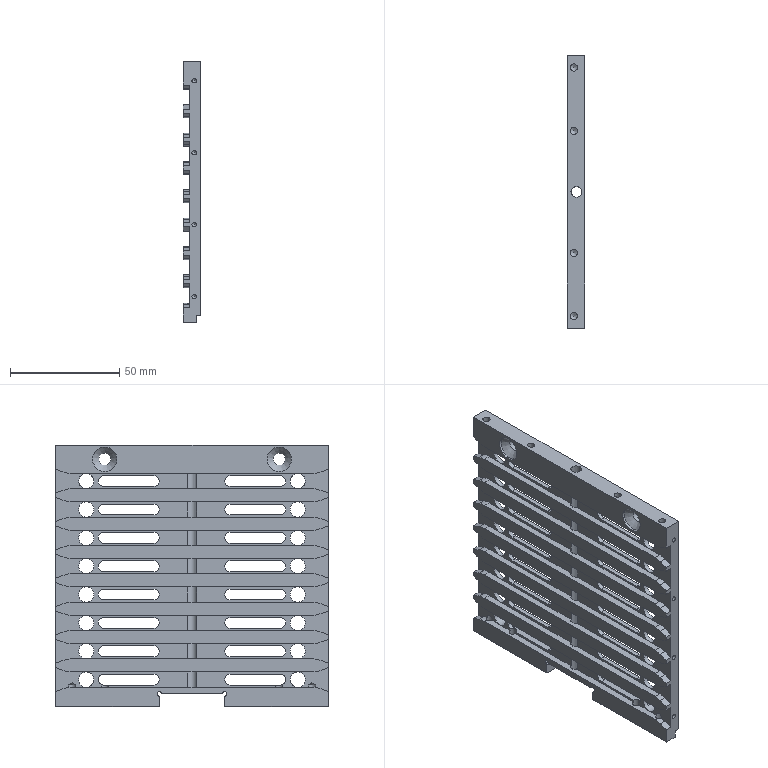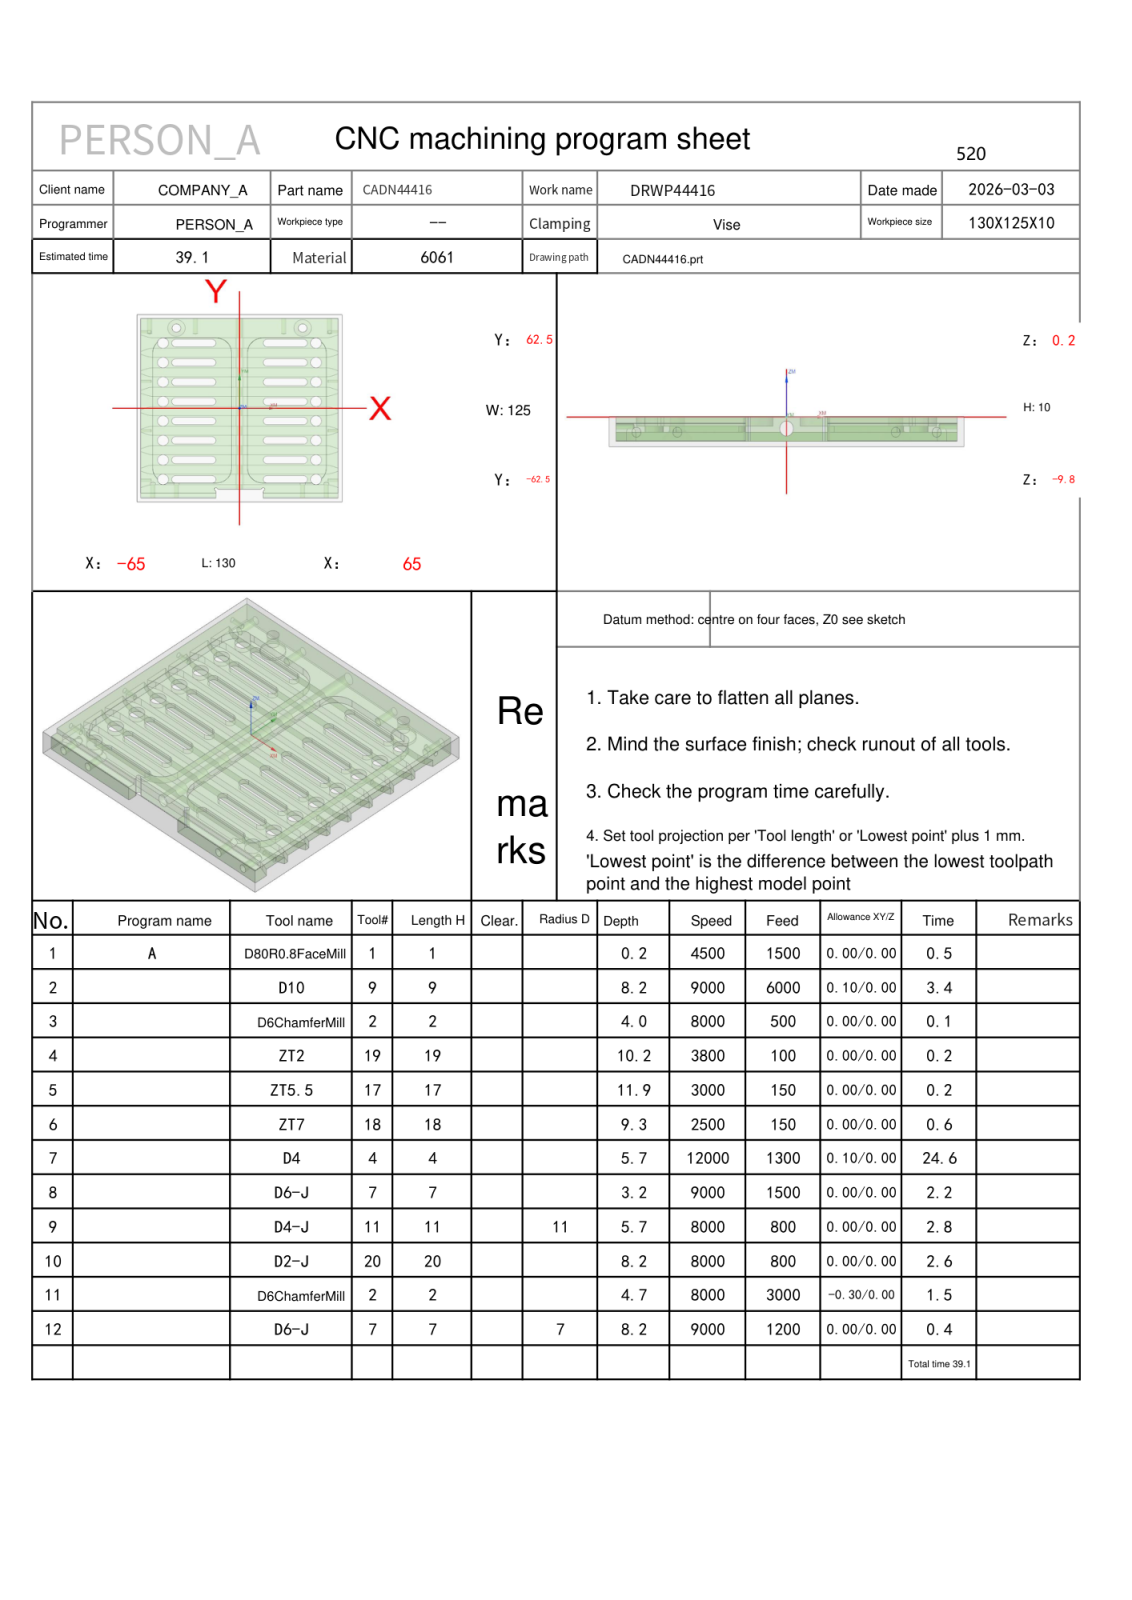NC program | NX | posted by the shop | part box 8 x 125 x 120 mm
Lines 826 to 1740 of 11100:
N7 T04 M06
(D4  D=4. R=0. H=04 ce=0.10 di=0.00)
G00 G90 G54 X29. Y-34.1 M03 S12000
G43 H04 Z30.
M08
Z-2.5
G01 X17.5 Z-2.536 F800.
G03 X17.1 Y-34.5 Z-2.538 I0.0 J-.4
X17.5 Y-34.9 Z-2.539 I.4 J0.0
G01 X40.5 Z-2.611
G03 X40.9 Y-34.5 Z-2.613 I0.0 J.4
X40.5 Y-34.1 Z-2.614 I-.4 J0.0
G01 X17.5 Z-2.686
G03 X17.1 Y-34.5 Z-2.688 I0.0 J-.4
X17.5 Y-34.9 Z-2.689 I.4 J0.0
G01 X40.5 Z-2.761
G03 X40.9 Y-34.5 Z-2.763 I0.0 J.4
X40.5 Y-34.1 Z-2.764 I-.4 J0.0
G01 X17.5 Z-2.836
G03 X17.1 Y-34.5 Z-2.838 I0.0 J-.4
X17.5 Y-34.9 Z-2.839 I.4 J0.0
G01 X40.5 Z-2.911
G03 X40.9 Y-34.5 Z-2.913 I0.0 J.4
X40.5 Y-34.1 Z-2.914 I-.4 J0.0
G01 X17.5 Z-2.986
G03 X17.1 Y-34.5 Z-2.988 I0.0 J-.4
X17.5 Y-34.9 Z-2.989 I.4 J0.0
G01 X40.5 Z-3.061
G03 X40.9 Y-34.5 Z-3.063 I0.0 J.4
X40.5 Y-34.1 Z-3.064 I-.4 J0.0
G01 X17.5 Z-3.136
G03 X17.1 Y-34.5 Z-3.138 I0.0 J-.4
X17.5 Y-34.9 Z-3.139 I.4 J0.0
G01 X40.5 Z-3.211
G03 X40.9 Y-34.5 Z-3.213 I0.0 J.4
X40.5 Y-34.1 Z-3.214 I-.4 J0.0
G01 X17.5 Z-3.286
G03 X17.1 Y-34.5 Z-3.288 I0.0 J-.4
X17.5 Y-34.9 Z-3.289 I.4 J0.0
G01 X40.5 Z-3.361
G03 X40.9 Y-34.5 Z-3.363 I0.0 J.4
X40.5 Y-34.1 Z-3.364 I-.4 J0.0
G01 X17.5 Z-3.436
G03 X17.1 Y-34.5 Z-3.438 I0.0 J-.4
X17.5 Y-34.9 Z-3.439 I.4 J0.0
G01 X40.5 Z-3.511
G03 X40.9 Y-34.5 Z-3.513 I0.0 J.4
X40.5 Y-34.1 Z-3.514 I-.4 J0.0
G01 X17.5 Z-3.586
G03 X17.1 Y-34.5 Z-3.588 I0.0 J-.4
X17.5 Y-34.9 Z-3.589 I.4 J0.0
G01 X40.5 Z-3.661
G03 X40.9 Y-34.5 Z-3.663 I0.0 J.4
X40.5 Y-34.1 Z-3.664 I-.4 J0.0
G01 X17.5 Z-3.736
G03 X17.1 Y-34.5 Z-3.738 I0.0 J-.4
X17.5 Y-34.9 Z-3.739 I.4 J0.0
G01 X40.5 Z-3.811
G03 X40.9 Y-34.5 Z-3.813 I0.0 J.4
X40.5 Y-34.1 Z-3.814 I-.4 J0.0
G01 X17.5 Z-3.886
G03 X17.1 Y-34.5 Z-3.888 I0.0 J-.4
X17.5 Y-34.9 Z-3.889 I.4 J0.0
G01 X40.5 Z-3.961
G03 X40.9 Y-34.5 Z-3.963 I0.0 J.4
X40.5 Y-34.1 Z-3.964 I-.4 J0.0
G01 X17.5 Z-4.036
G03 X17.1 Y-34.5 Z-4.038 I0.0 J-.4
X17.5 Y-34.9 Z-4.039 I.4 J0.0
G01 X40.5 Z-4.111
G03 X40.9 Y-34.5 Z-4.113 I0.0 J.4
X40.5 Y-34.1 Z-4.114 I-.4 J0.0
G01 X17.5 Z-4.186
G03 X17.1 Y-34.5 Z-4.188 I0.0 J-.4
X17.5 Y-34.9 Z-4.189 I.4 J0.0
G01 X40.5 Z-4.261
G03 X40.9 Y-34.5 Z-4.263 I0.0 J.4
X40.5 Y-34.1 Z-4.264 I-.4 J0.0
G01 X17.5 Z-4.336
G03 X17.1 Y-34.5 Z-4.338 I0.0 J-.4
X17.5 Y-34.9 Z-4.339 I.4 J0.0
G01 X40.5 Z-4.411
G03 X40.9 Y-34.5 Z-4.413 I0.0 J.4
X40.5 Y-34.1 Z-4.414 I-.4 J0.0
G01 X17.5 Z-4.486
G03 X17.1 Y-34.5 Z-4.488 I0.0 J-.4
X17.5 Y-34.9 Z-4.489 I.4 J0.0
G01 X40.5 Z-4.561
G03 X40.9 Y-34.5 Z-4.563 I0.0 J.4
X40.5 Y-34.1 Z-4.564 I-.4 J0.0
G01 X17.5 Z-4.636
G03 X17.1 Y-34.5 Z-4.638 I0.0 J-.4
X17.5 Y-34.9 Z-4.639 I.4 J0.0
G01 X40.5 Z-4.711
G03 X40.9 Y-34.5 Z-4.713 I0.0 J.4
X40.5 Y-34.1 Z-4.714 I-.4 J0.0
G01 X17.5 Z-4.786
G03 X17.1 Y-34.5 Z-4.788 I0.0 J-.4
X17.5 Y-34.9 Z-4.789 I.4 J0.0
G01 X40.5 Z-4.861
G03 X40.9 Y-34.5 Z-4.863 I0.0 J.4
X40.5 Y-34.1 Z-4.864 I-.4 J0.0
G01 X17.5 Z-4.936
G03 X17.1 Y-34.5 Z-4.938 I0.0 J-.4
X17.5 Y-34.9 Z-4.939 I.4 J0.0
G01 X40.5 Z-5.011
G03 X40.9 Y-34.5 Z-5.013 I0.0 J.4
X40.5 Y-34.1 Z-5.014 I-.4 J0.0
G01 X17.5 Z-5.086
G03 X17.1 Y-34.5 Z-5.088 I0.0 J-.4
X17.5 Y-34.9 Z-5.089 I.4 J0.0
G01 X40.5 Z-5.161
G03 X40.9 Y-34.5 Z-5.163 I0.0 J.4
X40.5 Y-34.1 Z-5.164 I-.4 J0.0
G01 X17.5 Z-5.236
G03 X17.1 Y-34.5 Z-5.238 I0.0 J-.4
X17.5 Y-34.9 Z-5.239 I.4 J0.0
G01 X40.5 Z-5.311
G03 X40.9 Y-34.5 Z-5.313 I0.0 J.4
X40.5 Y-34.1 Z-5.314 I-.4 J0.0
G01 X17.5 Z-5.386
G03 X17.1 Y-34.5 Z-5.388 I0.0 J-.4
X17.5 Y-34.9 Z-5.389 I.4 J0.0
G01 X40.5 Z-5.461
G03 X40.9 Y-34.5 Z-5.463 I0.0 J.4
X40.5 Y-34.1 Z-5.464 I-.4 J0.0
G01 X29. Z-5.5
X17.5
G03 X17.1 Y-34.5 I0.0 J-.4
X17.5 Y-34.9 I.4 J0.0
G01 X40.5
G03 X40.9 Y-34.5 I0.0 J.4
X40.5 Y-34.1 I-.4 J0.0
G01 X29.
X28.5
Z-4.5
G00 Z30.
X29. Y-21.9
Z-2.5
G01 X40.5 Z-2.536
G03 X40.9 Y-21.5 Z-2.538 I0.0 J.4
X40.5 Y-21.1 Z-2.539 I-.4 J0.0
G01 X17.5 Z-2.611
G03 X17.1 Y-21.5 Z-2.613 I0.0 J-.4
X17.5 Y-21.9 Z-2.614 I.4 J0.0
G01 X40.5 Z-2.686
G03 X40.9 Y-21.5 Z-2.688 I0.0 J.4
X40.5 Y-21.1 Z-2.689 I-.4 J0.0
G01 X17.5 Z-2.761
G03 X17.1 Y-21.5 Z-2.763 I0.0 J-.4
X17.5 Y-21.9 Z-2.764 I.4 J0.0
G01 X40.5 Z-2.836
G03 X40.9 Y-21.5 Z-2.838 I0.0 J.4
X40.5 Y-21.1 Z-2.839 I-.4 J0.0
G01 X17.5 Z-2.911
G03 X17.1 Y-21.5 Z-2.913 I0.0 J-.4
X17.5 Y-21.9 Z-2.914 I.4 J0.0
G01 X40.5 Z-2.986
G03 X40.9 Y-21.5 Z-2.988 I0.0 J.4
X40.5 Y-21.1 Z-2.989 I-.4 J0.0
G01 X17.5 Z-3.061
G03 X17.1 Y-21.5 Z-3.063 I0.0 J-.4
X17.5 Y-21.9 Z-3.064 I.4 J0.0
G01 X40.5 Z-3.136
G03 X40.9 Y-21.5 Z-3.138 I0.0 J.4
X40.5 Y-21.1 Z-3.139 I-.4 J0.0
G01 X17.5 Z-3.211
G03 X17.1 Y-21.5 Z-3.213 I0.0 J-.4
X17.5 Y-21.9 Z-3.214 I.4 J0.0
G01 X40.5 Z-3.286
G03 X40.9 Y-21.5 Z-3.288 I0.0 J.4
X40.5 Y-21.1 Z-3.289 I-.4 J0.0
G01 X17.5 Z-3.361
G03 X17.1 Y-21.5 Z-3.363 I0.0 J-.4
X17.5 Y-21.9 Z-3.364 I.4 J0.0
G01 X40.5 Z-3.436
G03 X40.9 Y-21.5 Z-3.438 I0.0 J.4
X40.5 Y-21.1 Z-3.439 I-.4 J0.0
G01 X17.5 Z-3.511
G03 X17.1 Y-21.5 Z-3.513 I0.0 J-.4
X17.5 Y-21.9 Z-3.514 I.4 J0.0
G01 X40.5 Z-3.586
G03 X40.9 Y-21.5 Z-3.588 I0.0 J.4
X40.5 Y-21.1 Z-3.589 I-.4 J0.0
G01 X17.5 Z-3.661
G03 X17.1 Y-21.5 Z-3.663 I0.0 J-.4
X17.5 Y-21.9 Z-3.664 I.4 J0.0
G01 X40.5 Z-3.736
G03 X40.9 Y-21.5 Z-3.738 I0.0 J.4
X40.5 Y-21.1 Z-3.739 I-.4 J0.0
G01 X17.5 Z-3.811
G03 X17.1 Y-21.5 Z-3.813 I0.0 J-.4
X17.5 Y-21.9 Z-3.814 I.4 J0.0
G01 X40.5 Z-3.886
G03 X40.9 Y-21.5 Z-3.888 I0.0 J.4
X40.5 Y-21.1 Z-3.889 I-.4 J0.0
G01 X17.5 Z-3.961
G03 X17.1 Y-21.5 Z-3.963 I0.0 J-.4
X17.5 Y-21.9 Z-3.964 I.4 J0.0
G01 X40.5 Z-4.036
G03 X40.9 Y-21.5 Z-4.038 I0.0 J.4
X40.5 Y-21.1 Z-4.039 I-.4 J0.0
G01 X17.5 Z-4.111
G03 X17.1 Y-21.5 Z-4.113 I0.0 J-.4
X17.5 Y-21.9 Z-4.114 I.4 J0.0
G01 X40.5 Z-4.186
G03 X40.9 Y-21.5 Z-4.188 I0.0 J.4
X40.5 Y-21.1 Z-4.189 I-.4 J0.0
G01 X17.5 Z-4.261
G03 X17.1 Y-21.5 Z-4.263 I0.0 J-.4
X17.5 Y-21.9 Z-4.264 I.4 J0.0
G01 X40.5 Z-4.336
G03 X40.9 Y-21.5 Z-4.338 I0.0 J.4
X40.5 Y-21.1 Z-4.339 I-.4 J0.0
G01 X17.5 Z-4.411
G03 X17.1 Y-21.5 Z-4.413 I0.0 J-.4
X17.5 Y-21.9 Z-4.414 I.4 J0.0
G01 X40.5 Z-4.486
G03 X40.9 Y-21.5 Z-4.488 I0.0 J.4
X40.5 Y-21.1 Z-4.489 I-.4 J0.0
G01 X17.5 Z-4.561
G03 X17.1 Y-21.5 Z-4.563 I0.0 J-.4
X17.5 Y-21.9 Z-4.564 I.4 J0.0
G01 X40.5 Z-4.636
G03 X40.9 Y-21.5 Z-4.638 I0.0 J.4
X40.5 Y-21.1 Z-4.639 I-.4 J0.0
G01 X17.5 Z-4.711
G03 X17.1 Y-21.5 Z-4.713 I0.0 J-.4
X17.5 Y-21.9 Z-4.714 I.4 J0.0
G01 X40.5 Z-4.786
G03 X40.9 Y-21.5 Z-4.788 I0.0 J.4
X40.5 Y-21.1 Z-4.789 I-.4 J0.0
G01 X17.5 Z-4.861
G03 X17.1 Y-21.5 Z-4.863 I0.0 J-.4
X17.5 Y-21.9 Z-4.864 I.4 J0.0
G01 X40.5 Z-4.936
G03 X40.9 Y-21.5 Z-4.938 I0.0 J.4
X40.5 Y-21.1 Z-4.939 I-.4 J0.0
G01 X17.5 Z-5.011
G03 X17.1 Y-21.5 Z-5.013 I0.0 J-.4
X17.5 Y-21.9 Z-5.014 I.4 J0.0
G01 X40.5 Z-5.086
G03 X40.9 Y-21.5 Z-5.088 I0.0 J.4
X40.5 Y-21.1 Z-5.089 I-.4 J0.0
G01 X17.5 Z-5.161
G03 X17.1 Y-21.5 Z-5.163 I0.0 J-.4
X17.5 Y-21.9 Z-5.164 I.4 J0.0
G01 X40.5 Z-5.236
G03 X40.9 Y-21.5 Z-5.238 I0.0 J.4
X40.5 Y-21.1 Z-5.239 I-.4 J0.0
G01 X17.5 Z-5.311
G03 X17.1 Y-21.5 Z-5.313 I0.0 J-.4
X17.5 Y-21.9 Z-5.314 I.4 J0.0
G01 X40.5 Z-5.386
G03 X40.9 Y-21.5 Z-5.388 I0.0 J.4
X40.5 Y-21.1 Z-5.389 I-.4 J0.0
G01 X17.5 Z-5.461
G03 X17.1 Y-21.5 Z-5.463 I0.0 J-.4
X17.5 Y-21.9 Z-5.464 I.4 J0.0
G01 X29. Z-5.5
X40.5
G03 X40.9 Y-21.5 I0.0 J.4
X40.5 Y-21.1 I-.4 J0.0
G01 X17.5
G03 X17.1 Y-21.5 I0.0 J-.4
X17.5 Y-21.9 I.4 J0.0
G01 X29.
X29.5
Z-4.5
G00 Z30.
X29. Y-8.9
Z-2.5
G01 X40.5 Z-2.536
G03 X40.9 Y-8.5 Z-2.538 I0.0 J.4
X40.5 Y-8.1 Z-2.539 I-.4 J0.0
G01 X17.5 Z-2.611
G03 X17.1 Y-8.5 Z-2.613 I0.0 J-.4
X17.5 Y-8.9 Z-2.614 I.4 J0.0
G01 X40.5 Z-2.686
G03 X40.9 Y-8.5 Z-2.688 I0.0 J.4
X40.5 Y-8.1 Z-2.689 I-.4 J0.0
G01 X17.5 Z-2.761
G03 X17.1 Y-8.5 Z-2.763 I0.0 J-.4
X17.5 Y-8.9 Z-2.764 I.4 J0.0
G01 X40.5 Z-2.836
G03 X40.9 Y-8.5 Z-2.838 I0.0 J.4
X40.5 Y-8.1 Z-2.839 I-.4 J0.0
G01 X17.5 Z-2.911
G03 X17.1 Y-8.5 Z-2.913 I0.0 J-.4
X17.5 Y-8.9 Z-2.914 I.4 J0.0
G01 X40.5 Z-2.986
G03 X40.9 Y-8.5 Z-2.988 I0.0 J.4
X40.5 Y-8.1 Z-2.989 I-.4 J0.0
G01 X17.5 Z-3.061
G03 X17.1 Y-8.5 Z-3.063 I0.0 J-.4
X17.5 Y-8.9 Z-3.064 I.4 J0.0
G01 X40.5 Z-3.136
G03 X40.9 Y-8.5 Z-3.138 I0.0 J.4
X40.5 Y-8.1 Z-3.139 I-.4 J0.0
G01 X17.5 Z-3.211
G03 X17.1 Y-8.5 Z-3.213 I0.0 J-.4
X17.5 Y-8.9 Z-3.214 I.4 J0.0
G01 X40.5 Z-3.286
G03 X40.9 Y-8.5 Z-3.288 I0.0 J.4
X40.5 Y-8.1 Z-3.289 I-.4 J0.0
G01 X17.5 Z-3.361
G03 X17.1 Y-8.5 Z-3.363 I0.0 J-.4
X17.5 Y-8.9 Z-3.364 I.4 J0.0
G01 X40.5 Z-3.436
G03 X40.9 Y-8.5 Z-3.438 I0.0 J.4
X40.5 Y-8.1 Z-3.439 I-.4 J0.0
G01 X17.5 Z-3.511
G03 X17.1 Y-8.5 Z-3.513 I0.0 J-.4
X17.5 Y-8.9 Z-3.514 I.4 J0.0
G01 X40.5 Z-3.586
G03 X40.9 Y-8.5 Z-3.588 I0.0 J.4
X40.5 Y-8.1 Z-3.589 I-.4 J0.0
G01 X17.5 Z-3.661
G03 X17.1 Y-8.5 Z-3.663 I0.0 J-.4
X17.5 Y-8.9 Z-3.664 I.4 J0.0
G01 X40.5 Z-3.736
G03 X40.9 Y-8.5 Z-3.738 I0.0 J.4
X40.5 Y-8.1 Z-3.739 I-.4 J0.0
G01 X17.5 Z-3.811
G03 X17.1 Y-8.5 Z-3.813 I0.0 J-.4
X17.5 Y-8.9 Z-3.814 I.4 J0.0
G01 X40.5 Z-3.886
G03 X40.9 Y-8.5 Z-3.888 I0.0 J.4
X40.5 Y-8.1 Z-3.889 I-.4 J0.0
G01 X17.5 Z-3.961
G03 X17.1 Y-8.5 Z-3.963 I0.0 J-.4
X17.5 Y-8.9 Z-3.964 I.4 J0.0
G01 X40.5 Z-4.036
G03 X40.9 Y-8.5 Z-4.038 I0.0 J.4
X40.5 Y-8.1 Z-4.039 I-.4 J0.0
G01 X17.5 Z-4.111
G03 X17.1 Y-8.5 Z-4.113 I0.0 J-.4
X17.5 Y-8.9 Z-4.114 I.4 J0.0
G01 X40.5 Z-4.186
G03 X40.9 Y-8.5 Z-4.188 I0.0 J.4
X40.5 Y-8.1 Z-4.189 I-.4 J0.0
G01 X17.5 Z-4.261
G03 X17.1 Y-8.5 Z-4.263 I0.0 J-.4
X17.5 Y-8.9 Z-4.264 I.4 J0.0
G01 X40.5 Z-4.336
G03 X40.9 Y-8.5 Z-4.338 I0.0 J.4
X40.5 Y-8.1 Z-4.339 I-.4 J0.0
G01 X17.5 Z-4.411
G03 X17.1 Y-8.5 Z-4.413 I0.0 J-.4
X17.5 Y-8.9 Z-4.414 I.4 J0.0
G01 X40.5 Z-4.486
G03 X40.9 Y-8.5 Z-4.488 I0.0 J.4
X40.5 Y-8.1 Z-4.489 I-.4 J0.0
G01 X17.5 Z-4.561
G03 X17.1 Y-8.5 Z-4.563 I0.0 J-.4
X17.5 Y-8.9 Z-4.564 I.4 J0.0
G01 X40.5 Z-4.636
G03 X40.9 Y-8.5 Z-4.638 I0.0 J.4
X40.5 Y-8.1 Z-4.639 I-.4 J0.0
G01 X17.5 Z-4.711
G03 X17.1 Y-8.5 Z-4.713 I0.0 J-.4
X17.5 Y-8.9 Z-4.714 I.4 J0.0
G01 X40.5 Z-4.786
G03 X40.9 Y-8.5 Z-4.788 I0.0 J.4
X40.5 Y-8.1 Z-4.789 I-.4 J0.0
G01 X17.5 Z-4.861
G03 X17.1 Y-8.5 Z-4.863 I0.0 J-.4
X17.5 Y-8.9 Z-4.864 I.4 J0.0
G01 X40.5 Z-4.936
G03 X40.9 Y-8.5 Z-4.938 I0.0 J.4
X40.5 Y-8.1 Z-4.939 I-.4 J0.0
G01 X17.5 Z-5.011
G03 X17.1 Y-8.5 Z-5.013 I0.0 J-.4
X17.5 Y-8.9 Z-5.014 I.4 J0.0
G01 X40.5 Z-5.086
G03 X40.9 Y-8.5 Z-5.088 I0.0 J.4
X40.5 Y-8.1 Z-5.089 I-.4 J0.0
G01 X17.5 Z-5.161
G03 X17.1 Y-8.5 Z-5.163 I0.0 J-.4
X17.5 Y-8.9 Z-5.164 I.4 J0.0
G01 X40.5 Z-5.236
G03 X40.9 Y-8.5 Z-5.238 I0.0 J.4
X40.5 Y-8.1 Z-5.239 I-.4 J0.0
G01 X17.5 Z-5.311
G03 X17.1 Y-8.5 Z-5.313 I0.0 J-.4
X17.5 Y-8.9 Z-5.314 I.4 J0.0
G01 X40.5 Z-5.386
G03 X40.9 Y-8.5 Z-5.388 I0.0 J.4
X40.5 Y-8.1 Z-5.389 I-.4 J0.0
G01 X17.5 Z-5.461
G03 X17.1 Y-8.5 Z-5.463 I0.0 J-.4
X17.5 Y-8.9 Z-5.464 I.4 J0.0
G01 X29. Z-5.5
X40.5
G03 X40.9 Y-8.5 I0.0 J.4
X40.5 Y-8.1 I-.4 J0.0
G01 X17.5
G03 X17.1 Y-8.5 I0.0 J-.4
X17.5 Y-8.9 I.4 J0.0
G01 X29.
X29.5
Z-4.5
G00 Z30.
X29. Y4.9
Z-2.5
G01 X17.5 Z-2.536
G03 X17.1 Y4.5 Z-2.538 I0.0 J-.4
X17.5 Y4.1 Z-2.539 I.4 J0.0
G01 X40.5 Z-2.611
G03 X40.9 Y4.5 Z-2.613 I0.0 J.4
X40.5 Y4.9 Z-2.614 I-.4 J0.0
G01 X17.5 Z-2.686
G03 X17.1 Y4.5 Z-2.688 I0.0 J-.4
X17.5 Y4.1 Z-2.689 I.4 J0.0
G01 X40.5 Z-2.761
G03 X40.9 Y4.5 Z-2.763 I0.0 J.4
X40.5 Y4.9 Z-2.764 I-.4 J0.0
G01 X17.5 Z-2.836
G03 X17.1 Y4.5 Z-2.838 I0.0 J-.4
X17.5 Y4.1 Z-2.839 I.4 J0.0
G01 X40.5 Z-2.911
G03 X40.9 Y4.5 Z-2.913 I0.0 J.4
X40.5 Y4.9 Z-2.914 I-.4 J0.0
G01 X17.5 Z-2.986
G03 X17.1 Y4.5 Z-2.988 I0.0 J-.4
X17.5 Y4.1 Z-2.989 I.4 J0.0
G01 X40.5 Z-3.061
G03 X40.9 Y4.5 Z-3.063 I0.0 J.4
X40.5 Y4.9 Z-3.064 I-.4 J0.0
G01 X17.5 Z-3.136
G03 X17.1 Y4.5 Z-3.138 I0.0 J-.4
X17.5 Y4.1 Z-3.139 I.4 J0.0
G01 X40.5 Z-3.211
G03 X40.9 Y4.5 Z-3.213 I0.0 J.4
X40.5 Y4.9 Z-3.214 I-.4 J0.0
G01 X17.5 Z-3.286
G03 X17.1 Y4.5 Z-3.288 I0.0 J-.4
X17.5 Y4.1 Z-3.289 I.4 J0.0
G01 X40.5 Z-3.361
G03 X40.9 Y4.5 Z-3.363 I0.0 J.4
X40.5 Y4.9 Z-3.364 I-.4 J0.0
G01 X17.5 Z-3.436
G03 X17.1 Y4.5 Z-3.438 I0.0 J-.4
X17.5 Y4.1 Z-3.439 I.4 J0.0
G01 X40.5 Z-3.511
G03 X40.9 Y4.5 Z-3.513 I0.0 J.4
X40.5 Y4.9 Z-3.514 I-.4 J0.0
G01 X17.5 Z-3.586
G03 X17.1 Y4.5 Z-3.588 I0.0 J-.4
X17.5 Y4.1 Z-3.589 I.4 J0.0
G01 X40.5 Z-3.661
G03 X40.9 Y4.5 Z-3.663 I0.0 J.4
X40.5 Y4.9 Z-3.664 I-.4 J0.0
G01 X17.5 Z-3.736
G03 X17.1 Y4.5 Z-3.738 I0.0 J-.4
X17.5 Y4.1 Z-3.739 I.4 J0.0
G01 X40.5 Z-3.811
G03 X40.9 Y4.5 Z-3.813 I0.0 J.4
X40.5 Y4.9 Z-3.814 I-.4 J0.0
G01 X17.5 Z-3.886
G03 X17.1 Y4.5 Z-3.888 I0.0 J-.4
X17.5 Y4.1 Z-3.889 I.4 J0.0
G01 X40.5 Z-3.961
G03 X40.9 Y4.5 Z-3.963 I0.0 J.4
X40.5 Y4.9 Z-3.964 I-.4 J0.0
G01 X17.5 Z-4.036
G03 X17.1 Y4.5 Z-4.038 I0.0 J-.4
X17.5 Y4.1 Z-4.039 I.4 J0.0
G01 X40.5 Z-4.111
G03 X40.9 Y4.5 Z-4.113 I0.0 J.4
X40.5 Y4.9 Z-4.114 I-.4 J0.0
G01 X17.5 Z-4.186
G03 X17.1 Y4.5 Z-4.188 I0.0 J-.4
X17.5 Y4.1 Z-4.189 I.4 J0.0
G01 X40.5 Z-4.261
G03 X40.9 Y4.5 Z-4.263 I0.0 J.4
X40.5 Y4.9 Z-4.264 I-.4 J0.0
G01 X17.5 Z-4.336
G03 X17.1 Y4.5 Z-4.338 I0.0 J-.4
X17.5 Y4.1 Z-4.339 I.4 J0.0
G01 X40.5 Z-4.411
G03 X40.9 Y4.5 Z-4.413 I0.0 J.4
X40.5 Y4.9 Z-4.414 I-.4 J0.0
G01 X17.5 Z-4.486
G03 X17.1 Y4.5 Z-4.488 I0.0 J-.4
X17.5 Y4.1 Z-4.489 I.4 J0.0
G01 X40.5 Z-4.561
G03 X40.9 Y4.5 Z-4.563 I0.0 J.4
X40.5 Y4.9 Z-4.564 I-.4 J0.0
G01 X17.5 Z-4.636
G03 X17.1 Y4.5 Z-4.638 I0.0 J-.4
X17.5 Y4.1 Z-4.639 I.4 J0.0
G01 X40.5 Z-4.711
G03 X40.9 Y4.5 Z-4.713 I0.0 J.4
X40.5 Y4.9 Z-4.714 I-.4 J0.0
G01 X17.5 Z-4.786
G03 X17.1 Y4.5 Z-4.788 I0.0 J-.4
X17.5 Y4.1 Z-4.789 I.4 J0.0
G01 X40.5 Z-4.861
G03 X40.9 Y4.5 Z-4.863 I0.0 J.4
X40.5 Y4.9 Z-4.864 I-.4 J0.0
G01 X17.5 Z-4.936
G03 X17.1 Y4.5 Z-4.938 I0.0 J-.4
X17.5 Y4.1 Z-4.939 I.4 J0.0
G01 X40.5 Z-5.011
G03 X40.9 Y4.5 Z-5.013 I0.0 J.4
X40.5 Y4.9 Z-5.014 I-.4 J0.0
G01 X17.5 Z-5.086
G03 X17.1 Y4.5 Z-5.088 I0.0 J-.4
X17.5 Y4.1 Z-5.089 I.4 J0.0
G01 X40.5 Z-5.161
G03 X40.9 Y4.5 Z-5.163 I0.0 J.4
X40.5 Y4.9 Z-5.164 I-.4 J0.0
G01 X17.5 Z-5.236
G03 X17.1 Y4.5 Z-5.238 I0.0 J-.4
X17.5 Y4.1 Z-5.239 I.4 J0.0
G01 X40.5 Z-5.311
G03 X40.9 Y4.5 Z-5.313 I0.0 J.4
X40.5 Y4.9 Z-5.314 I-.4 J0.0
G01 X17.5 Z-5.386
G03 X17.1 Y4.5 Z-5.388 I0.0 J-.4
X17.5 Y4.1 Z-5.389 I.4 J0.0
G01 X40.5 Z-5.461
G03 X40.9 Y4.5 Z-5.463 I0.0 J.4
X40.5 Y4.9 Z-5.464 I-.4 J0.0
G01 X29. Z-5.5
X17.5
G03 X17.1 Y4.5 I0.0 J-.4
X17.5 Y4.1 I.4 J0.0
G01 X40.5
G03 X40.9 Y4.5 I0.0 J.4
X40.5 Y4.9 I-.4 J0.0
G01 X29.
X28.5
Z-4.5
G00 Z30.
X29. Y17.1
Z-2.5
G01 X40.5 Z-2.536
G03 X40.9 Y17.5 Z-2.538 I0.0 J.4
X40.5 Y17.9 Z-2.539 I-.4 J0.0
G01 X17.5 Z-2.611
G03 X17.1 Y17.5 Z-2.613 I0.0 J-.4
X17.5 Y17.1 Z-2.614 I.4 J0.0
G01 X40.5 Z-2.686
G03 X40.9 Y17.5 Z-2.688 I0.0 J.4
X40.5 Y17.9 Z-2.689 I-.4 J0.0
G01 X17.5 Z-2.761
G03 X17.1 Y17.5 Z-2.763 I0.0 J-.4
X17.5 Y17.1 Z-2.764 I.4 J0.0
G01 X40.5 Z-2.836
G03 X40.9 Y17.5 Z-2.838 I0.0 J.4
X40.5 Y17.9 Z-2.839 I-.4 J0.0
G01 X17.5 Z-2.911
G03 X17.1 Y17.5 Z-2.913 I0.0 J-.4
X17.5 Y17.1 Z-2.914 I.4 J0.0
G01 X40.5 Z-2.986
G03 X40.9 Y17.5 Z-2.988 I0.0 J.4
X40.5 Y17.9 Z-2.989 I-.4 J0.0
G01 X17.5 Z-3.061
G03 X17.1 Y17.5 Z-3.063 I0.0 J-.4
X17.5 Y17.1 Z-3.064 I.4 J0.0
G01 X40.5 Z-3.136
G03 X40.9 Y17.5 Z-3.138 I0.0 J.4
X40.5 Y17.9 Z-3.139 I-.4 J0.0
G01 X17.5 Z-3.211
G03 X17.1 Y17.5 Z-3.213 I0.0 J-.4
X17.5 Y17.1 Z-3.214 I.4 J0.0
G01 X40.5 Z-3.286
G03 X40.9 Y17.5 Z-3.288 I0.0 J.4
X40.5 Y17.9 Z-3.289 I-.4 J0.0
G01 X17.5 Z-3.361
G03 X17.1 Y17.5 Z-3.363 I0.0 J-.4
X17.5 Y17.1 Z-3.364 I.4 J0.0
G01 X40.5 Z-3.436
G03 X40.9 Y17.5 Z-3.438 I0.0 J.4
X40.5 Y17.9 Z-3.439 I-.4 J0.0
G01 X17.5 Z-3.511
G03 X17.1 Y17.5 Z-3.513 I0.0 J-.4
X17.5 Y17.1 Z-3.514 I.4 J0.0
G01 X40.5 Z-3.586
G03 X40.9 Y17.5 Z-3.588 I0.0 J.4
X40.5 Y17.9 Z-3.589 I-.4 J0.0
G01 X17.5 Z-3.661
G03 X17.1 Y17.5 Z-3.663 I0.0 J-.4
X17.5 Y17.1 Z-3.664 I.4 J0.0
G01 X40.5 Z-3.736
G03 X40.9 Y17.5 Z-3.738 I0.0 J.4
X40.5 Y17.9 Z-3.739 I-.4 J0.0
G01 X17.5 Z-3.811
G03 X17.1 Y17.5 Z-3.813 I0.0 J-.4
X17.5 Y17.1 Z-3.814 I.4 J0.0
G01 X40.5 Z-3.886
G03 X40.9 Y17.5 Z-3.888 I0.0 J.4
X40.5 Y17.9 Z-3.889 I-.4 J0.0
G01 X17.5 Z-3.961
G03 X17.1 Y17.5 Z-3.963 I0.0 J-.4
X17.5 Y17.1 Z-3.964 I.4 J0.0
G01 X40.5 Z-4.036
G03 X40.9 Y17.5 Z-4.038 I0.0 J.4
X40.5 Y17.9 Z-4.039 I-.4 J0.0
G01 X17.5 Z-4.111
G03 X17.1 Y17.5 Z-4.113 I0.0 J-.4
X17.5 Y17.1 Z-4.114 I.4 J0.0
G01 X40.5 Z-4.186
G03 X40.9 Y17.5 Z-4.188 I0.0 J.4
X40.5 Y17.9 Z-4.189 I-.4 J0.0
G01 X17.5 Z-4.261
G03 X17.1 Y17.5 Z-4.263 I0.0 J-.4
X17.5 Y17.1 Z-4.264 I.4 J0.0
G01 X40.5 Z-4.336
G03 X40.9 Y17.5 Z-4.338 I0.0 J.4
X40.5 Y17.9 Z-4.339 I-.4 J0.0
G01 X17.5 Z-4.411
G03 X17.1 Y17.5 Z-4.413 I0.0 J-.4
X17.5 Y17.1 Z-4.414 I.4 J0.0
G01 X40.5 Z-4.486
G03 X40.9 Y17.5 Z-4.488 I0.0 J.4
X40.5 Y17.9 Z-4.489 I-.4 J0.0
G01 X17.5 Z-4.561
G03 X17.1 Y17.5 Z-4.563 I0.0 J-.4
X17.5 Y17.1 Z-4.564 I.4 J0.0
G01 X40.5 Z-4.636
G03 X40.9 Y17.5 Z-4.638 I0.0 J.4
X40.5 Y17.9 Z-4.639 I-.4 J0.0
G01 X17.5 Z-4.711
G03 X17.1 Y17.5 Z-4.713 I0.0 J-.4
X17.5 Y17.1 Z-4.714 I.4 J0.0
G01 X40.5 Z-4.786
G03 X40.9 Y17.5 Z-4.788 I0.0 J.4
X40.5 Y17.9 Z-4.789 I-.4 J0.0
G01 X17.5 Z-4.861
G03 X17.1 Y17.5 Z-4.863 I0.0 J-.4
X17.5 Y17.1 Z-4.864 I.4 J0.0
G01 X40.5 Z-4.936
G03 X40.9 Y17.5 Z-4.938 I0.0 J.4
X40.5 Y17.9 Z-4.939 I-.4 J0.0
G01 X17.5 Z-5.011
G03 X17.1 Y17.5 Z-5.013 I0.0 J-.4
X17.5 Y17.1 Z-5.014 I.4 J0.0
G01 X40.5 Z-5.086
G03 X40.9 Y17.5 Z-5.088 I0.0 J.4
X40.5 Y17.9 Z-5.089 I-.4 J0.0
G01 X17.5 Z-5.161
G03 X17.1 Y17.5 Z-5.163 I0.0 J-.4
X17.5 Y17.1 Z-5.164 I.4 J0.0
G01 X40.5 Z-5.236
G03 X40.9 Y17.5 Z-5.238 I0.0 J.4
X40.5 Y17.9 Z-5.239 I-.4 J0.0
G01 X17.5 Z-5.311
G03 X17.1 Y17.5 Z-5.313 I0.0 J-.4
X17.5 Y17.1 Z-5.314 I.4 J0.0
G01 X40.5 Z-5.386
G03 X40.9 Y17.5 Z-5.388 I0.0 J.4
X40.5 Y17.9 Z-5.389 I-.4 J0.0
G01 X17.5 Z-5.461
G03 X17.1 Y17.5 Z-5.463 I0.0 J-.4
X17.5 Y17.1 Z-5.464 I.4 J0.0
G01 X29. Z-5.5
X40.5
G03 X40.9 Y17.5 I0.0 J.4
X40.5 Y17.9 I-.4 J0.0
G01 X17.5
G03 X17.1 Y17.5 I0.0 J-.4
X17.5 Y17.1 I.4 J0.0
G01 X29.
X29.5
Z-4.5
G00 Z30.
X29. Y30.1
Z-2.5
G01 X40.5 Z-2.536
G03 X40.9 Y30.5 Z-2.538 I0.0 J.4
X40.5 Y30.9 Z-2.539 I-.4 J0.0
G01 X17.5 Z-2.611
G03 X17.247 Y30.81 Z-2.611 I0.0 J-.4
X17.1 Y30.5 Z-2.613 I.253 J-.31
X17.5 Y30.1 Z-2.614 I.4 J0.0
G01 X40.5 Z-2.686
G03 X40.9 Y30.5 Z-2.688 I0.0 J.4
X40.5 Y30.9 Z-2.689 I-.4 J0.0
G01 X17.5 Z-2.761
G03 X17.247 Y30.81 Z-2.761 I0.0 J-.4
X17.1 Y30.5 Z-2.763 I.253 J-.31
X17.5 Y30.1 Z-2.764 I.4 J0.0
G01 X40.5 Z-2.836
G03 X40.9 Y30.5 Z-2.838 I0.0 J.4
X40.5 Y30.9 Z-2.839 I-.4 J0.0
G01 X17.5 Z-2.911
G03 X17.247 Y30.81 Z-2.911 I0.0 J-.4
X17.1 Y30.5 Z-2.913 I.253 J-.31
X17.5 Y30.1 Z-2.914 I.4 J0.0
G01 X40.5 Z-2.986
G03 X40.9 Y30.5 Z-2.988 I0.0 J.4
X40.5 Y30.9 Z-2.989 I-.4 J0.0
G01 X17.5 Z-3.061
G03 X17.247 Y30.81 Z-3.061 I0.0 J-.4
X17.1 Y30.5 Z-3.063 I.253 J-.31
X17.5 Y30.1 Z-3.064 I.4 J0.0
G01 X40.5 Z-3.136
G03 X40.9 Y30.5 Z-3.138 I0.0 J.4
X40.5 Y30.9 Z-3.139 I-.4 J0.0
G01 X17.5 Z-3.211
G03 X17.247 Y30.81 Z-3.211 I0.0 J-.4
X17.1 Y30.5 Z-3.213 I.253 J-.31
X17.5 Y30.1 Z-3.214 I.4 J0.0
G01 X40.5 Z-3.286
G03 X40.9 Y30.5 Z-3.288 I0.0 J.4
X40.5 Y30.9 Z-3.289 I-.4 J0.0
G01 X17.5 Z-3.361
G03 X17.247 Y30.81 Z-3.361 I0.0 J-.4
X17.1 Y30.5 Z-3.363 I.253 J-.31
X17.5 Y30.1 Z-3.364 I.4 J0.0
G01 X40.5 Z-3.436
G03 X40.9 Y30.5 Z-3.438 I0.0 J.4
X40.5 Y30.9 Z-3.439 I-.4 J0.0
G01 X17.5 Z-3.511
G03 X17.247 Y30.81 Z-3.511 I0.0 J-.4
X17.1 Y30.5 Z-3.513 I.253 J-.31
X17.5 Y30.1 Z-3.514 I.4 J0.0
G01 X40.5 Z-3.586
G03 X40.9 Y30.5 Z-3.588 I0.0 J.4
X40.5 Y30.9 Z-3.589 I-.4 J0.0
G01 X17.5 Z-3.661
G03 X17.247 Y30.81 Z-3.661 I0.0 J-.4
X17.1 Y30.5 Z-3.663 I.253 J-.31
X17.5 Y30.1 Z-3.664 I.4 J0.0
G01 X40.5 Z-3.736
G03 X40.9 Y30.5 Z-3.738 I0.0 J.4
X40.5 Y30.9 Z-3.739 I-.4 J0.0
G01 X17.5 Z-3.811
G03 X17.247 Y30.81 Z-3.811 I0.0 J-.4
X17.1 Y30.5 Z-3.813 I.253 J-.31
X17.5 Y30.1 Z-3.814 I.4 J0.0
G01 X40.5 Z-3.886
G03 X40.9 Y30.5 Z-3.888 I0.0 J.4
X40.5 Y30.9 Z-3.889 I-.4 J0.0
G01 X17.5 Z-3.961
G03 X17.247 Y30.81 Z-3.961 I0.0 J-.4
X17.1 Y30.5 Z-3.963 I.253 J-.31
X17.5 Y30.1 Z-3.964 I.4 J0.0
G01 X40.5 Z-4.036
G03 X40.9 Y30.5 Z-4.038 I0.0 J.4
X40.5 Y30.9 Z-4.039 I-.4 J0.0
G01 X17.5 Z-4.111
G03 X17.247 Y30.81 Z-4.111 I0.0 J-.4
X17.1 Y30.5 Z-4.113 I.253 J-.31
X17.5 Y30.1 Z-4.114 I.4 J0.0
G01 X40.5 Z-4.186
G03 X40.9 Y30.5 Z-4.188 I0.0 J.4
X40.5 Y30.9 Z-4.189 I-.4 J0.0
G01 X17.5 Z-4.261
G03 X17.247 Y30.81 Z-4.261 I0.0 J-.4
X17.1 Y30.5 Z-4.263 I.253 J-.31
X17.5 Y30.1 Z-4.264 I.4 J0.0
G01 X40.5 Z-4.336
G03 X40.9 Y30.5 Z-4.338 I0.0 J.4
X40.5 Y30.9 Z-4.339 I-.4 J0.0
G01 X17.5 Z-4.411
G03 X17.247 Y30.81 Z-4.411 I0.0 J-.4
X17.1 Y30.5 Z-4.413 I.253 J-.31
X17.5 Y30.1 Z-4.414 I.4 J0.0
G01 X40.5 Z-4.486
G03 X40.9 Y30.5 Z-4.488 I0.0 J.4
X40.5 Y30.9 Z-4.489 I-.4 J0.0
G01 X17.5 Z-4.561
G03 X17.247 Y30.81 Z-4.561 I0.0 J-.4
X17.1 Y30.5 Z-4.563 I.253 J-.31
X17.5 Y30.1 Z-4.564 I.4 J0.0
G01 X40.5 Z-4.636
G03 X40.9 Y30.5 Z-4.638 I0.0 J.4
X40.5 Y30.9 Z-4.639 I-.4 J0.0
G01 X17.5 Z-4.711
G03 X17.247 Y30.81 Z-4.711 I0.0 J-.4
X17.1 Y30.5 Z-4.713 I.253 J-.31
X17.5 Y30.1 Z-4.714 I.4 J0.0
G01 X40.5 Z-4.786
G03 X40.9 Y30.5 Z-4.788 I0.0 J.4
X40.5 Y30.9 Z-4.789 I-.4 J0.0
G01 X17.5 Z-4.861
G03 X17.247 Y30.81 Z-4.861 I0.0 J-.4
X17.1 Y30.5 Z-4.863 I.253 J-.31
X17.5 Y30.1 Z-4.864 I.4 J0.0
G01 X40.5 Z-4.936
G03 X40.9 Y30.5 Z-4.938 I0.0 J.4
X40.5 Y30.9 Z-4.939 I-.4 J0.0
G01 X17.5 Z-5.011
G03 X17.247 Y30.81 Z-5.011 I0.0 J-.4
X17.1 Y30.5 Z-5.013 I.253 J-.31
X17.5 Y30.1 Z-5.014 I.4 J0.0
G01 X40.5 Z-5.086
G03 X40.9 Y30.5 Z-5.088 I0.0 J.4
X40.5 Y30.9 Z-5.089 I-.4 J0.0
G01 X17.5 Z-5.161
G03 X17.247 Y30.81 Z-5.161 I0.0 J-.4
X17.1 Y30.5 Z-5.163 I.253 J-.31
X17.5 Y30.1 Z-5.164 I.4 J0.0
G01 X40.5 Z-5.236
G03 X40.9 Y30.5 Z-5.238 I0.0 J.4
X40.5 Y30.9 Z-5.239 I-.4 J0.0
G01 X17.5 Z-5.311
G03 X17.247 Y30.81 Z-5.311 I0.0 J-.4
X17.1 Y30.5 Z-5.313 I.253 J-.31
X17.5 Y30.1 Z-5.314 I.4 J0.0
G01 X40.5 Z-5.386
G03 X40.9 Y30.5 Z-5.388 I0.0 J.4
X40.5 Y30.9 Z-5.389 I-.4 J0.0
G01 X17.5 Z-5.461
G03 X17.247 Y30.81 Z-5.461 I0.0 J-.4
X17.1 Y30.5 Z-5.463 I.253 J-.31
X17.5 Y30.1 Z-5.464 I.4 J0.0
G01 X29. Z-5.5
X40.5
G03 X40.9 Y30.5 I0.0 J.4
X40.5 Y30.9 I-.4 J0.0
G01 X17.5
G03 X17.1 Y30.5 I0.0 J-.4
X17.5 Y30.1 I.4 J0.0
G01 X29.
X29.5
Z-4.5
G00 Z30.
X29. Y43.1
Z-2.5
G01 X40.5 Z-2.536
G03 X40.753 Y43.19 Z-2.536 I0.0 J.4
X40.9 Y43.5 Z-2.538 I-.253 J.31
X40.5 Y43.9 Z-2.539 I-.4 J0.0
G01 X17.5 Z-2.611
G03 X17.1 Y43.5 Z-2.613 I0.0 J-.4
X17.247 Y43.19 Z-2.614 I.4 J0.0
X17.5 Y43.1 Z-2.614 I.253 J.31
G01 X40.5 Z-2.686
G03 X40.753 Y43.19 Z-2.686 I0.0 J.4
X40.9 Y43.5 Z-2.688 I-.253 J.31
X40.5 Y43.9 Z-2.689 I-.4 J0.0
G01 X17.5 Z-2.761
G03 X17.1 Y43.5 Z-2.763 I0.0 J-.4
X17.247 Y43.19 Z-2.764 I.4 J0.0
X17.5 Y43.1 Z-2.764 I.253 J.31
G01 X40.5 Z-2.836
G03 X40.753 Y43.19 Z-2.836 I0.0 J.4
X40.9 Y43.5 Z-2.838 I-.253 J.31
X40.5 Y43.9 Z-2.839 I-.4 J0.0
G01 X17.5 Z-2.911
G03 X17.1 Y43.5 Z-2.913 I0.0 J-.4
X17.247 Y43.19 Z-2.914 I.4 J0.0
X17.5 Y43.1 Z-2.914 I.253 J.31
G01 X40.5 Z-2.986
G03 X40.753 Y43.19 Z-2.986 I0.0 J.4
X40.9 Y43.5 Z-2.988 I-.253 J.31
X40.5 Y43.9 Z-2.989 I-.4 J0.0
G01 X17.5 Z-3.061
G03 X17.1 Y43.5 Z-3.063 I0.0 J-.4
X17.247 Y43.19 Z-3.064 I.4 J0.0
X17.5 Y43.1 Z-3.064 I.253 J.31
G01 X40.5 Z-3.136
G03 X40.753 Y43.19 Z-3.136 I0.0 J.4
X40.9 Y43.5 Z-3.138 I-.253 J.31
X40.5 Y43.9 Z-3.139 I-.4 J0.0
G01 X17.5 Z-3.211
G03 X17.1 Y43.5 Z-3.213 I0.0 J-.4
X17.247 Y43.19 Z-3.214 I.4 J0.0
X17.5 Y43.1 Z-3.214 I.253 J.31
G01 X40.5 Z-3.286
G03 X40.753 Y43.19 Z-3.286 I0.0 J.4
X40.9 Y43.5 Z-3.288 I-.253 J.31
X40.5 Y43.9 Z-3.289 I-.4 J0.0
G01 X17.5 Z-3.361
G03 X17.1 Y43.5 Z-3.363 I0.0 J-.4
X17.247 Y43.19 Z-3.364 I.4 J0.0
X17.5 Y43.1 Z-3.364 I.253 J.31
G01 X40.5 Z-3.436
G03 X40.753 Y43.19 Z-3.436 I0.0 J.4
X40.9 Y43.5 Z-3.438 I-.253 J.31
X40.5 Y43.9 Z-3.439 I-.4 J0.0
G01 X17.5 Z-3.511
G03 X17.1 Y43.5 Z-3.513 I0.0 J-.4
X17.247 Y43.19 Z-3.514 I.4 J0.0
X17.5 Y43.1 Z-3.514 I.253 J.31
G01 X40.5 Z-3.586
G03 X40.753 Y43.19 Z-3.586 I0.0 J.4
X40.9 Y43.5 Z-3.588 I-.253 J.31
X40.5 Y43.9 Z-3.589 I-.4 J0.0
G01 X17.5 Z-3.661
G03 X17.1 Y43.5 Z-3.663 I0.0 J-.4
X17.247 Y43.19 Z-3.664 I.4 J0.0
X17.5 Y43.1 Z-3.664 I.253 J.31
G01 X40.5 Z-3.736
G03 X40.753 Y43.19 Z-3.736 I0.0 J.4
X40.9 Y43.5 Z-3.738 I-.253 J.31
X40.5 Y43.9 Z-3.739 I-.4 J0.0
G01 X17.5 Z-3.811
G03 X17.1 Y43.5 Z-3.813 I0.0 J-.4
X17.247 Y43.19 Z-3.814 I.4 J0.0
X17.5 Y43.1 Z-3.814 I.253 J.31
G01 X40.5 Z-3.886
G03 X40.753 Y43.19 Z-3.886 I0.0 J.4
X40.9 Y43.5 Z-3.888 I-.253 J.31
X40.5 Y43.9 Z-3.889 I-.4 J0.0
G01 X17.5 Z-3.961
G03 X17.1 Y43.5 Z-3.963 I0.0 J-.4
X17.247 Y43.19 Z-3.964 I.4 J0.0
X17.5 Y43.1 Z-3.964 I.253 J.31
G01 X40.5 Z-4.036
G03 X40.753 Y43.19 Z-4.036 I0.0 J.4
X40.9 Y43.5 Z-4.038 I-.253 J.31
X40.5 Y43.9 Z-4.039 I-.4 J0.0
G01 X17.5 Z-4.111
G03 X17.1 Y43.5 Z-4.113 I0.0 J-.4
X17.247 Y43.19 Z-4.114 I.4 J0.0
X17.5 Y43.1 Z-4.114 I.253 J.31
G01 X40.5 Z-4.186
G03 X40.753 Y43.19 Z-4.186 I0.0 J.4
X40.9 Y43.5 Z-4.188 I-.253 J.31